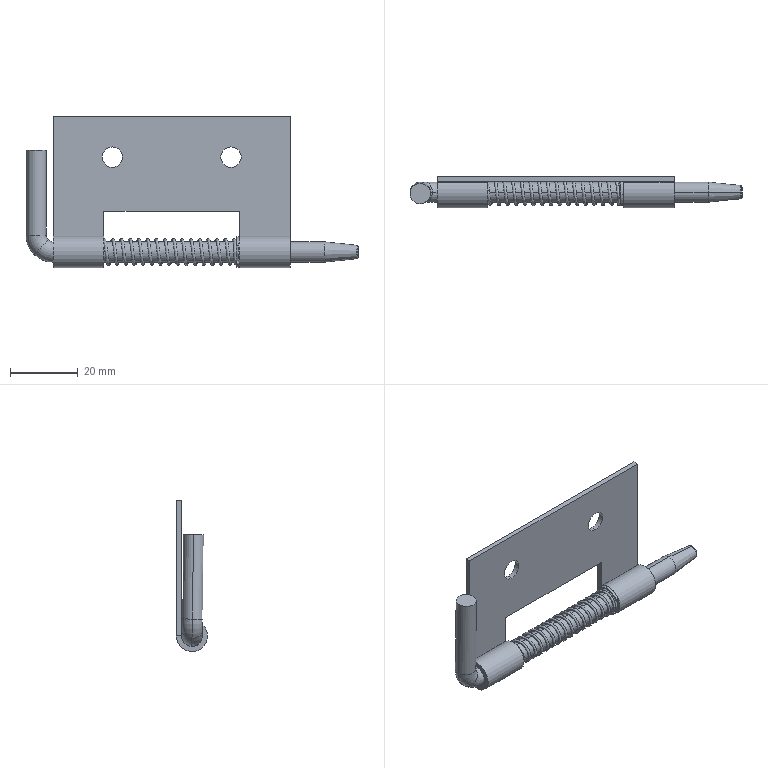Part | NX | features BREP 4 | 4 solids | 74 faces | box 98 x 9.2 x 44.6 mm | volume 7933 mm3 | cylinder 32 | plane 28 | torus 8 | spline 4 | cone 2 | commonest cylinder face diameters 6 x10 0.8 x7 4 x6 9 x3 6.2 x2 6.4 x2